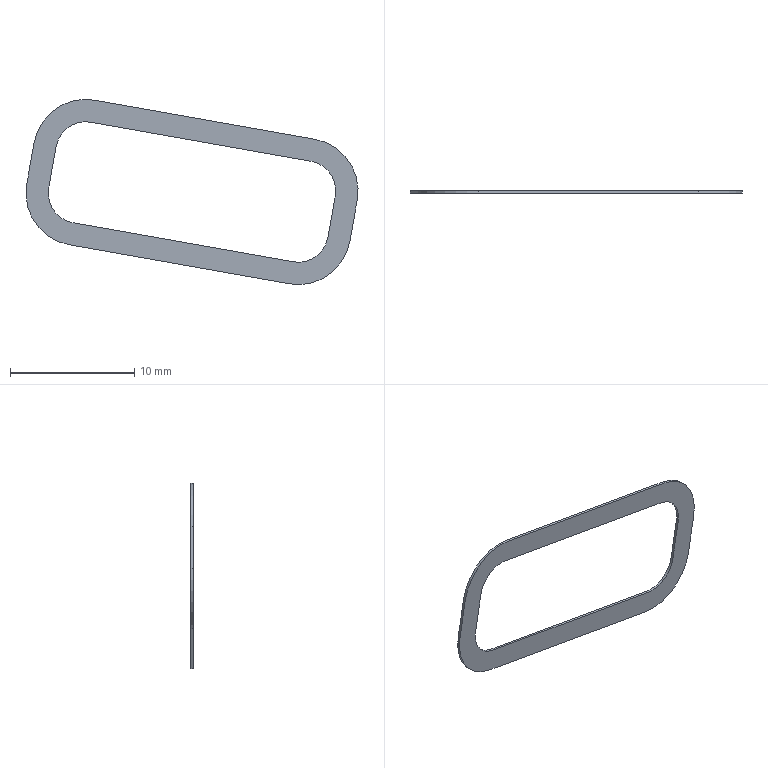Part | SolidWorks | features BaseBody 1 | 1 solid | 20 faces | box 26.743 x 0.2 x 14.919 mm | volume 22.901 mm3 | cylinder 10 | plane 10 | commonest cylinder face diameters 8.425 x6 4.825 x4